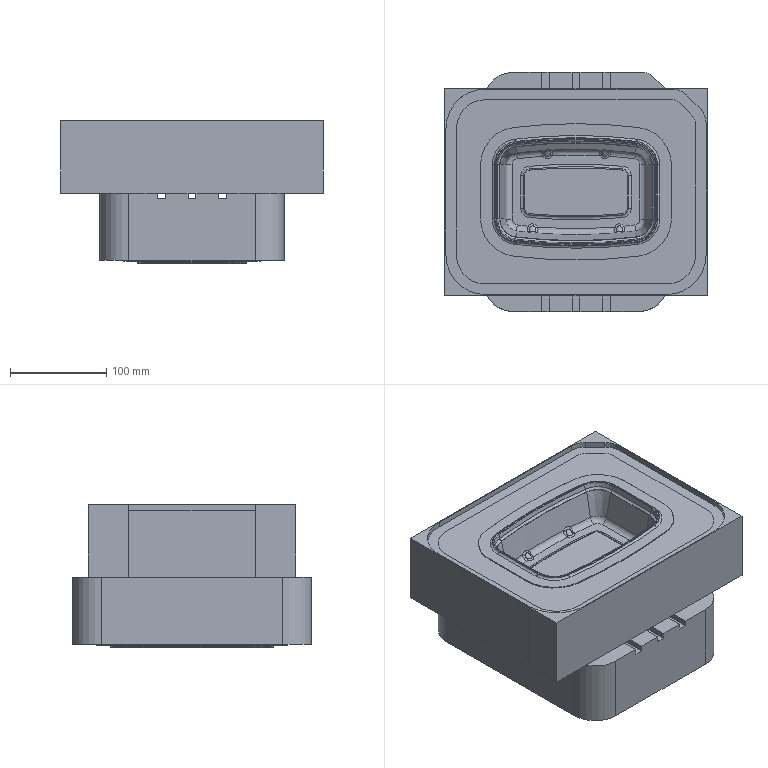NC program | NX | posted with a generic post | part box 272.387 x 248.388 x 148.5 mm
Lines 5839 to 6739 of 133013:
(CONTOUR_AREA_1 , TOOL : R2)
N11676 M6
N11678 G53
N11680 G17 G0 G90 X-11.083 Y-70.672 S8000 M3 M8
N11682 G43 Z133. H0
N11684 Z73.707
N11686 G94 G1 Z70.707 F4500.
N11688 X-11.776 Y-70.653
N11690 X-12.469 Y-70.629
N11692 X-13.16 Y-70.612
N11694 X-21.466 Y-70.357
N11696 X-22.535 Y-70.31
N11698 X-32.555 Y-69.794
N11700 X-33.592 Y-69.724
N11702 X-41.216 Y-69.179
N11704 X-43.287 Y-69.03
N11706 G3 X-50.565 Y-68.366 R5781.693
N11708 G1 X-54.029 Y-68.047
N11710 X-57.148 Y-67.701
N11712 X-64.761 Y-66.846
N11714 X-64.768 Y-66.841
N11716 X-65.111 Y-66.795
N11718 X-66.981 Y-66.5
N11720 X-67.876 Y-66.349
N11722 X-68.74 Y-66.153
N11724 X-70.174 Y-65.808
N11726 X-70.653 Y-65.686
N11728 X-70.998 Y-65.589
N11730 X-71.419 Y-65.461
N11732 X-71.695 Y-65.369
N11734 X-73.556 Y-64.768
N11736 X-73.771 Y-64.686
N11738 X-74.397 Y-64.432
N11740 X-74.812 Y-64.261
N11742 X-76.116 Y-63.729
N11744 X-76.539 Y-63.537
N11746 X-78.925 Y-62.343
N11748 X-79.525 Y-61.997
N11750 X-79.661 Y-61.916
N11752 X-81.252 Y-60.958
N11754 X-81.793 Y-60.612
N11756 X-83.741 Y-59.226
N11758 X-84.196 Y-58.88
N11760 X-84.856 Y-58.331
N11762 X-86.279 Y-57.148
N11764 X-88.419 Y-55.07
N11766 X-90.396 Y-52.834
N11768 X-92.129 Y-50.551
N11770 X-92.821 Y-49.485
N11772 X-93.237 Y-48.836
N11774 X-93.681 Y-48.143
N11776 X-93.888 Y-47.796
N11778 X-95.008 Y-45.718
N11780 X-95.189 Y-45.372
N11782 X-95.242 Y-45.265
N11784 X-96.285 Y-42.931
N11786 X-96.421 Y-42.601
N11788 X-96.551 Y-42.255
N11790 X-97.29 Y-40.177
N11792 X-97.322 Y-40.086
N11794 X-97.406 Y-39.831
N11796 X-97.6 Y-39.138
N11798 X-97.979 Y-37.752
N11800 X-98.162 Y-37.06
N11802 X-98.364 Y-36.069
N11804 X-98.707 Y-34.289
N11806 X-98.725 Y-34.247
N11808 X-99.073 Y-31.172
N11810 X-99.17 Y-28.747
N11812 X-99.189 Y-27.715
N11814 Y28.048
N11816 X-99.158 Y29.09
N11818 X-99.075 Y31.125
N11820 X-99.071 Y31.172
N11822 X-99.056 Y31.321
N11824 X-98.878 Y32.904
N11826 X-98.725 Y34.247
N11828 X-98.707 Y34.289
N11830 X-98.364 Y36.068
N11832 X-98.162 Y37.06
N11834 X-98.072 Y37.406
N11836 X-97.979 Y37.752
N11838 X-97.406 Y39.831
N11840 X-97.171 Y40.513
N11842 X-96.672 Y41.909
N11844 X-96.55 Y42.255
N11846 X-96.424 Y42.595
N11848 X-96.285 Y42.931
N11850 X-95.814 Y43.989
N11852 X-95.351 Y45.026
N11854 X-95.246 Y45.258
N11856 X-95.19 Y45.372
N11858 X-95.008 Y45.719
N11860 X-94.821 Y46.065
N11862 X-93.861 Y47.845
N11864 X-93.682 Y48.142
N11866 X-93.459 Y48.489
N11868 X-92.345 Y50.221
N11870 X-92.129 Y50.55
N11872 X-90.397 Y52.833
N11874 X-89.012 Y54.399
N11876 X-88.419 Y55.07
N11878 X-86.934 Y56.512
N11880 X-86.241 Y57.179
N11882 X-84.163 Y58.906
N11884 X-83.741 Y59.226
N11886 X-83.253 Y59.573
N11888 X-81.739 Y60.649
N11890 X-81.251 Y60.958
N11892 X-81.045 Y61.082
N11894 X-80.007 Y61.705
N11896 X-79.314 Y62.121
N11898 X-78.924 Y62.344
N11900 X-76.543 Y63.535
N11902 X-76.257 Y63.665
N11904 X-76.116 Y63.729
N11906 X-74.812 Y64.261
N11908 X-74.119 Y64.546
N11910 X-73.773 Y64.683
N11912 X-73.556 Y64.768
N11914 X-71.348 Y65.482
N11916 X-71.002 Y65.588
N11918 X-70.656 Y65.686
N11920 X-70.179 Y65.807
N11922 X-69.963 Y65.858
N11924 X-69.292 Y66.018
N11926 X-68.584 Y66.19
N11928 X-67.885 Y66.347
N11930 X-66.159 Y66.63
N11932 X-65.46 Y66.742
N11934 X-65.114 Y66.795
N11936 X-64.768 Y66.841
N11938 X-64.76 Y66.846
N11940 X-61.65 Y67.192
N11942 X-60.265 Y67.349
N11944 X-55.432 Y67.894
N11946 X-54.031 Y68.046
N11948 X-53.338 Y68.111
N11950 X-45.802 Y68.802
N11952 X-44.501 Y68.924
N11954 X-44.333 Y68.937
N11956 X-43.294 Y69.03
N11958 X-33.596 Y69.724
N11960 X-32.557 Y69.794
N11962 X-29.107 Y69.973
N11964 X-22.534 Y70.308
N11966 X-21.474 Y70.357
N11968 X-11.776 Y70.653
N11970 X-11.743 Y70.656
N11972 X-10.737 Y70.68
N11974 X-0.346 Y70.786
N11976 X0.
N11978 X0.345
N11980 X1.732 Y70.773
N11982 X3.803 Y70.751
N11984 X5.542 Y70.733
N11986 X6.927 Y70.721
N11988 X10.707 Y70.681
N11990 G2 X40.869 Y69.204 R522.773
N11992 G1 X43.287 Y69.03
N11994 G2 X53.684 Y68.08 R1157.552
N11996 G1 X54.377 Y68.01
N11998 X59.226 Y67.466
N12000 X60.954 Y67.273
N12002 X61.997 Y67.157
N12004 X62.688 Y67.078
N12006 X63.382 Y66.998
N12008 X64.761 Y66.846
N12010 X64.768 Y66.841
N12012 X65.111 Y66.795
N12014 X65.805 Y66.688
N12016 X66.5 Y66.576
N12018 X66.981 Y66.5
N12020 X67.876 Y66.349
N12022 X68.74 Y66.153
N12024 X70.174 Y65.808
N12026 X70.653 Y65.686
N12028 X70.998 Y65.589
N12030 X71.419 Y65.461
N12032 X73.556 Y64.768
N12034 X74.667 Y64.32
N12036 G2 X79.661 Y61.916 R33.441
N12038 G1 X81.252 Y60.958
N12040 X81.39 Y60.87
N12042 X81.793 Y60.612
N12044 X83.741 Y59.226
N12046 X83.817 Y59.168
N12048 X84.196 Y58.88
N12050 X85.862 Y57.495
N12052 X86.279 Y57.148
N12054 X88.419 Y55.07
N12056 X88.725 Y54.724
N12058 X90.396 Y52.834
N12060 X90.79 Y52.317
N12062 X92.129 Y50.551
N12064 X92.346 Y50.221
N12066 X92.79 Y49.532
N12068 X92.822 Y49.485
N12070 X93.237 Y48.836
N12072 X93.681 Y48.143
N12074 X93.888 Y47.796
N12076 X93.964 Y47.656 Z70.705
N12078 X94.072 Y47.455 Z70.707
N12080 X95.008 Y45.719
N12082 X95.19 Y45.372
N12084 X95.243 Y45.265
N12086 X96.285 Y42.931
N12088 X96.421 Y42.601
N12090 X96.551 Y42.255
N12092 X97.168 Y40.523
N12094 X97.406 Y39.831
N12096 X98.162 Y37.06
N12098 X98.364 Y36.069
N12100 X98.707 Y34.289
N12102 X98.725 Y34.247
N12104 X99.073 Y31.172
N12106 X99.158 Y29.094
N12108 X99.189 Y28.055
N12110 X99.185 Y-28.055
N12112 G2 X99.056 Y-31.321 R74.044
N12114 G1 X98.725 Y-34.247
N12116 X98.707 Y-34.289
N12118 X98.364 Y-36.068
N12120 X98.162 Y-37.06
N12122 X98.087 Y-37.352
N12124 X97.672 Y-38.88
N12126 X97.409 Y-39.821
N12128 X97.244 Y-40.311
N12130 X96.672 Y-41.909
N12132 X96.634 Y-42.021
N12134 X96.424 Y-42.595
N12136 X96.285 Y-42.931
N12138 X95.815 Y-43.987
N12140 X95.244 Y-45.262
N12142 X95.189 Y-45.372
N12144 X95.008 Y-45.719
N12146 X94.822 Y-46.065
N12148 X93.888 Y-47.796
N12150 X93.682 Y-48.142
N12152 X93.459 Y-48.489
N12154 X92.568 Y-49.875
N12156 X92.129 Y-50.55
N12158 X92.115 Y-50.568
N12160 X91.783 Y-51.006
N12162 X91.437 Y-51.464
N12164 X90.803 Y-52.299
N12166 X90.397 Y-52.833
N12168 X89.358 Y-54.008
N12170 X88.421 Y-55.067
N12172 X86.279 Y-57.148
N12174 X85.862 Y-57.495
N12176 G2 X81.392 Y-60.871 R37.735
N12178 G1 X79.526 Y-61.994
N12180 X78.925 Y-62.343
N12182 X76.543 Y-63.535
N12184 X76.115 Y-63.729
N12186 X73.773 Y-64.685
N12188 X73.556 Y-64.768
N12190 X72.045 Y-65.255
N12192 X71.43 Y-65.457
N12194 X71.002 Y-65.588
N12196 X70.656 Y-65.686
N12198 X70.18 Y-65.806
N12200 X68.931 Y-66.106
N12202 X68.745 Y-66.152
N12204 X67.885 Y-66.347
N12206 X66.983 Y-66.499
N12208 X66.5 Y-66.576
N12210 X65.807 Y-66.688
N12212 X65.114 Y-66.795
N12214 X64.768 Y-66.841
N12216 X64.76 Y-66.846
N12218 X61.65 Y-67.192
N12220 X60.958 Y-67.272
N12222 X59.919 Y-67.387
N12224 X59.226 Y-67.467
N12226 X58.187 Y-67.582
N12228 X57.494 Y-67.662
N12230 X56.455 Y-67.777
N12232 X55.869 Y-67.845
N12234 X55.52 Y-67.884
N12236 X54.377 Y-68.01
N12238 X53.684 Y-68.08
N12240 X44.333 Y-68.937
N12242 X43.294 Y-69.03
N12244 X42.601 Y-69.079
N12246 X32.903 Y-69.773
N12248 X29.44 Y-69.957
N12250 X25.284 Y-70.168
N12252 X24.591 Y-70.201
N12254 X23.898 Y-70.238
N12256 X22.874 Y-70.289
N12258 X22.534 Y-70.31
N12260 X21.474 Y-70.357
N12262 X11.43 Y-70.663
N12264 X10.737 Y-70.68
N12266 X10.506 Y-70.683
N12268 X8.659 Y-70.703
N12270 X0.347 Y-70.786
N12272 X-1.039 Y-70.78
N12274 X-10.737 Y-70.679
N12276 X-11.083 Y-70.672
N12278 Y-70.387
N12280 X-21.577 Y-70.067
N12282 X-22.513 Y-70.025
N12284 X-32.557 Y-69.508
N12286 X-39.83 Y-68.993
N12288 X-40.148 Y-68.971
N12290 X-41.186 Y-68.895
N12292 X-43.446 Y-68.73
N12294 X-45.986 Y-68.499
N12296 X-54.031 Y-67.759
N12298 X-56.027 Y-67.539
N12300 X-60.148 Y-67.076
N12302 X-61.393 Y-66.935
N12304 X-61.713 Y-66.902
N12306 G2 X-68.087 Y-66.009 R64.071
N12308 X-73.663 Y-64.422 R39.26
N12310 G1 X-74.223 Y-64.194
N12312 X-74.725 Y-63.989
N12314 G2 X-79.548 Y-61.651 R33.299
N12316 X-91.914 Y-50.358 R38.49
N12318 G1 X-92.605 Y-49.295
N12320 G2 X-96.529 Y-41.46 R35.482
N12322 G1 X-96.985 Y-40.189
N12324 X-97.081 Y-39.907
N12326 G2 X-98.214 Y-35.328 R35.034
N12328 G1 X-98.416 Y-34.289
N12330 X-98.459 Y-34.035
N12332 X-98.472 Y-33.943
N12334 X-98.784 Y-31.172
N12336 X-98.889 Y-28.58
N12338 X-98.904 Y-27.902
N12340 X-98.902 Y28.055
N12342 X-98.865 Y29.285
N12344 X-98.783 Y31.203
N12346 X-98.46 Y34.036
N12348 G2 X-97.081 Y39.901 R40.617
N12350 G1 X-96.978 Y40.198
N12352 X-96.802 Y40.7
N12354 G2 X-94.125 Y46.758 R33.961
N12356 G1 X-93.62 Y47.692
N12358 X-93.286 Y48.231
N12360 X-91.919 Y50.351
N12362 G2 X-70.33 Y65.474 R38.676
N12364 G1 X-70.019 Y65.551
N12366 X-69.371 Y65.707
N12368 G2 X-64.51 Y66.587 R34.841
N12370 G1 X-61.657 Y66.907
N12372 X-61.583 Y66.914
N12374 X-61.304 Y66.945
N12376 G2 X-36.401 Y69.237 R453.922
N12378 G1 X-35.328 Y69.315
N12380 X-34.981 Y69.339
N12382 X-32.557 Y69.508
N12384 G2 X10.82 Y70.393 R533.867
N12386 G1 X15.273 Y70.262
N12388 G2 X39.57 Y69.011 R454.953
N12390 G1 X40.148 Y68.971
N12392 X40.523 Y68.943
N12394 G2 X61.713 Y66.902 R454.097
N12396 G1 X62.023 Y66.867
N12398 X63.382 Y66.711
N12400 G2 X67.885 Y66.054 R50.215
N12402 X76.431 Y63.27 R39.532
N12404 X91.917 Y50.354 R38.732
N12406 G1 X92.605 Y49.295
N12408 G2 X98.148 Y35.674 R37.937
N12410 G1 X98.417 Y34.289
N12412 X98.46 Y34.036
N12414 X98.784 Y31.172
N12416 X98.878 Y28.915
N12418 X98.904 Y27.902
N12420 X98.902 Y-28.055
N12422 X98.877 Y-28.926
N12424 X98.783 Y-31.203
N12426 X98.459 Y-34.035
N12428 G2 X96.221 Y-42.32 R40.059
N12430 X92.228 Y-49.875 R37.191
N12432 G1 X91.919 Y-50.351
N12434 X90.179 Y-52.646
N12436 X88.326 Y-54.745
N12438 X88.003 Y-55.079
N12440 X87.656 Y-55.416
N12442 G2 X74.517 Y-64.075 R37.871
N12444 G1 X74.224 Y-64.195
N12446 X73.663 Y-64.422
N12448 X73.426 Y-64.51
N12450 X72.459 Y-64.823
N12452 X71.76 Y-65.049
N12454 X71.364 Y-65.179
N12456 X71.248 Y-65.214
N12458 X70.656 Y-65.388
N12460 X70.385 Y-65.461
N12462 X70.331 Y-65.475
N12464 X70.02 Y-65.551
N12466 X68.577 Y-65.898
N12468 G2 X64.51 Y-66.587 R37.613
N12470 G1 X61.657 Y-66.907
N12472 X61.582 Y-66.914
N12474 X60.958 Y-66.985
N12476 G2 X40.544 Y-68.941 R450.136
N12478 G1 X40.177 Y-68.969
N12480 X39.757 Y-68.997
N12482 X32.674 Y-69.5
N12484 X28.747 Y-69.705
N12486 X22.903 Y-70.002
N12488 X22.517 Y-70.025
N12490 X21.82 Y-70.056
N12492 X20.781 Y-70.091
N12494 X12.843 Y-70.334
N12496 X10.65 Y-70.396
N12498 X0. Y-70.502
N12500 X-10.82 Y-70.393
N12502 X-11.083 Y-70.387
N12504 Y-70.102
N12506 X-21.636 Y-69.779
N12508 X-23.552 Y-69.685
N12510 X-32.512 Y-69.225
N12512 X-40.177 Y-68.683
N12514 X-43.501 Y-68.439
N12516 X-44.679 Y-68.335
N12518 X-54.031 Y-67.473
N12520 X-57.089 Y-67.134
N12522 X-64.56 Y-66.292
N12524 G2 X-73.521 Y-64.17 R41.197
N12526 X-91.658 Y-50.221 R38.444
N12528 G1 X-92.338 Y-49.182
N12530 X-93.202 Y-47.831
N12532 X-93.515 Y-47.288
N12534 X-94.665 Y-45.148
N12536 X-95.308 Y-43.724
N12538 G2 X-98.125 Y-34.289 R37.617
N12540 G1 X-98.161 Y-34.086
N12542 G2 X-98.618 Y-27.963 R40.788
N12544 G1 X-98.615 Y28.149
N12546 G2 X-98.46 Y31.518 R77.107
N12548 X-97.539 Y37.192 R35.328
N12550 X-95.701 Y42.84 R39.307
N12552 X-92.56 Y48.836 R36.752
N12554 X-85.895 Y56.712 R37.84
N12556 X-65.039 Y66.229 R38.365
N12558 G1 X-64.639 Y66.282
N12560 G2 X10.88 Y70.106 R532.641
N12562 G1 X15.288 Y69.976
N12564 X21.636 Y69.779
N12566 G2 X43.294 Y68.456 R559.26
N12568 G1 X45.994 Y68.213
N12570 G2 X65.114 Y66.218 R500.357
N12572 X70.309 Y65.185 R37.681
N12574 X73.521 Y64.17 R32.159
N12576 X93.515 Y47.287 R38.331
N12578 X98.591 Y28.974 R38.203
N12580 G1 X98.618 Y27.963
N12582 X98.616 Y-28.149
N12584 X98.586 Y-29.094
N12586 G2 X97.538 Y-37.192 R36.316
N12588 X93.305 Y-47.66 R38.64
N12590 X89.799 Y-52.646 R39.677
N12592 X86.173 Y-56.456 R37.052
N12594 X65.039 Y-66.228 R38.449
N12596 G1 X64.639 Y-66.282
N12598 G2 X0.092 Y-70.217 R540.463
N12600 G1 X-8.659 Y-70.133
N12602 X-11.083 Y-70.102
N12604 X-11.076 Y-69.817
N12606 X-21.694 Y-69.491
N12608 X-29.786 Y-69.082
N12610 X-32.555 Y-68.937
N12612 X-43.238 Y-68.175
N12614 X-44.829 Y-68.035
N12616 X-53.973 Y-67.192
N12618 X-58.533 Y-66.685
N12620 X-64.612 Y-65.998
N12622 G2 X-73.546 Y-63.854 R38.916
N12624 X-91.504 Y-49.942 R38.116
N12626 G1 X-92.129 Y-48.98
N12628 G2 X-97.528 Y-35.878 R37.067
N12630 X-98.333 Y-28.024 R38.449
N12632 G1 X-98.332 Y28.086
N12634 X-98.312 Y28.747
N12636 G2 X-96.433 Y40.029 R37.083
N12638 X-64.571 Y66.003 R38.089
N12640 X43.294 Y68.171 R532.489
N12642 G1 X46.097 Y67.917
N12644 X53.682 Y67.221
N12646 X55.416 Y67.036
N12648 X64.612 Y65.998
N12650 G2 X73.546 Y63.854 R38.887
N12652 X91.437 Y50.042 R38.131
N12654 G1 X92.129 Y48.98
N12656 G2 X97.528 Y35.878 R37.056
N12658 X98.323 Y28.401 R37.333
N12660 G1 X98.333 Y28.024
N12662 X98.332 Y-28.086
N12664 X98.324 Y-28.401
N12666 X98.312 Y-28.799
N12668 G2 X97.893 Y-33.943 R40.122
N12670 G1 X97.871 Y-34.089
N12672 X97.457 Y-36.234
N12674 G2 X92.129 Y-48.98 R37.548
N12676 G1 X91.437 Y-50.038
N12678 G2 X87.973 Y-54.278 R40.986
N12680 X64.571 Y-66.003 R38.122
N12682 X29.44 Y-69.101 R523.114
N12684 X10.527 Y-69.827 R478.814
N12686 G1 X0.03 Y-69.933
N12688 X-10.6 Y-69.826
N12690 X-10.94 Y-69.82
N12692 X-11.076 Y-69.817
N12694 X-11.068 Y-69.532
N12696 X-21.42 Y-69.217
N12698 G2 X-58.442 Y-66.409 R514.424
N12700 G1 X-64.421 Y-65.735
N12702 G2 X-75.64 Y-62.69 R38.52
N12704 X-91.204 Y-49.875 R37.832
N12706 G1 X-91.883 Y-48.836
N12708 G2 X-97.277 Y-35.674 R36.78
N12710 G1 X-97.565 Y-34.183
N12712 X-97.607 Y-33.943
N12714 G2 X-98.047 Y-28.089 R39.97
N12716 G1 X-98.048 Y28.021
N12718 G2 X-97.913 Y31.276 R45.935
N12720 X-96.467 Y38.956 R35.912
N12722 G1 X-96.33 Y39.44
N12724 G2 X-95.246 Y42.453 R73.943
N12726 X-89.63 Y51.953 R38.041
N12728 X-73.651 Y63.504 R37.754
N12730 X-64.503 Y65.725 R38.644
N12732 X13.693 Y69.455 R530.504
N12734 X46.755 Y67.57 R495.456
N12736 X65.27 Y65.617 R434.821
N12738 X97.565 Y34.183 R37.729
N12740 G1 X97.607 Y33.943
N12742 X97.616 Y33.887
N12744 X97.923 Y31.172
N12746 X97.949 Y30.757
N12748 X98.017 Y29.094
N12750 X98.047 Y28.089
N12752 X98.049 Y-28.02
N12754 G2 X97.913 Y-31.276 R46.903
N12756 X96.466 Y-38.957 R38.469
N12758 X92.962 Y-47.104 R36.701
N12760 G1 X92.822 Y-47.354
N12762 G2 X91.09 Y-50.03 R71.844
N12764 X64.503 Y-65.725 R37.832
N12766 X22.257 Y-69.18 R538.667
N12768 G1 X21.531 Y-69.213
N12770 G2 X-11.068 Y-69.532 R537.912
N12772 G1 X-11.06 Y-69.247
N12774 X-21.473 Y-68.93
N12776 X-23.461 Y-68.833
N12778 X-32.356 Y-68.377
N12780 X-35.272 Y-68.176
N12782 G2 X-58.496 Y-66.116 R486.59
N12784 G1 X-64.41 Y-65.45
N12786 G2 X-78.318 Y-61.047 R38.223
N12788 X-93.906 Y-44.75 R37.454
N12790 G1 X-94.563 Y-43.294
N12792 G2 X-96.978 Y-35.721 R35.934
N12794 G1 X-97.324 Y-33.91
N12796 X-97.642 Y-31.143
N12798 G2 X-97.762 Y-28.055 R103.283
N12800 G1 Y28.055
N12802 G2 X-97.635 Y31.208 R95.138
N12804 X-96.71 Y36.982 R35.154
N12806 G1 X-96.119 Y39.138
N12808 X-96.052 Y39.371
N12810 G2 X-95.019 Y42.255 R77.519
N12812 X-73.023 Y63.44 R37.639
N12814 X-64.318 Y65.461 R39.061
N12816 X10.721 Y69.255 R532.311
N12818 G1 X15.325 Y69.12
N12820 G2 X45.573 Y67.393 R504.84
N12822 G1 X53.818 Y66.634
N12824 X55.382 Y66.466
N12826 X64.41 Y65.45
N12828 G2 X78.275 Y61.07 R38.206
N12830 X97.36 Y33.632 R37.453
N12832 G1 X97.5 Y32.402
N12834 G2 X97.74 Y28.817 R25.703
N12836 G1 X97.76 Y28.144
N12838 X97.762 Y28.055
N12840 Y-28.055
N12842 G2 X96.71 Y-36.982 R38.006
N12844 X81.046 Y-59.388 R37.45
N12846 X64.835 Y-65.394 R37.73
N12848 X29.49 Y-68.528 R513.606
N12850 G1 X22.193 Y-68.898
N12852 G2 X-11.06 Y-69.247 R528.151
N12854 G1 X-11.081 Y-68.961
N12856 X-21.474 Y-68.645
N12858 G2 X-54.031 Y-66.326 R535.764
N12860 G1 X-58.531 Y-65.825
N12862 X-64.42 Y-65.161
N12864 G2 X-73.102 Y-63.109 R39.742
N12866 X-90.744 Y-49.539 R37.29
N12868 X-93.622 Y-44.68 R40.427
N12870 X-96.684 Y-35.738 R36.386
N12872 X-97.464 Y-28.541 R34.735
N12874 G1 X-97.478 Y-27.862
N12876 X-97.476 Y28.055
N12878 X-97.437 Y29.328
N12880 G2 X-97.04 Y33.88 R32.842
N12882 X-90.978 Y49.182 R37.588
N12884 X-87.356 Y53.685 R37.229
N12886 X-65.173 Y65.056 R37.142
N12888 G1 X-64.368 Y65.168
N12890 G2 X-32.719 Y68.069 R537.621
N12892 G1 X-26.508 Y68.393
N12894 X-22.13 Y68.615
N12896 X-21.474 Y68.645
N12898 G2 X10.735 Y68.97 R532.128
N12900 G1 X15.215 Y68.838
N12902 X21.474 Y68.645
N12904 G2 X55.414 Y66.175 R532.578
N12906 G1 X64.42 Y65.161
N12908 G2 X75.352 Y62.191 R37.931
N12910 X90.744 Y49.54 R37.378
N12912 X93.622 Y44.68 R40.53
N12914 X97.476 Y28.055 R37.734
N12916 G1 X97.477 Y-28.055
N12918 G2 X97.04 Y-33.881 R40.605
N12920 X89.012 Y-51.806 R37.234
N12922 X82.731 Y-57.841 R37.953
N12924 X77.87 Y-60.958 R36.322
N12926 X65.173 Y-65.055 R37.121
N12928 G1 X64.368 Y-65.167
N12930 G2 X29.442 Y-68.245 R515.836
N12932 X10.739 Y-68.97 R469.788
N12934 G1 X0. Y-69.077
N12936 X-10.735 Y-68.97
N12938 X-11.081 Y-68.961
N12940 X-11.083 Y-68.676
N12942 X-21.596 Y-68.354
N12944 X-29.785 Y-67.94
N12946 X-32.796 Y-67.778
N12948 X-42.818 Y-67.063
N12950 X-43.46 Y-67.012
N12952 X-53.927 Y-66.05
N12954 X-58.533 Y-65.538
N12956 X-64.514 Y-64.861
N12958 G2 X-77.922 Y-60.612 R37.297
N12960 X-97.177 Y-28.6 R36.873
N12962 G1 X-97.193 Y-27.923
N12964 X-97.191 Y28.055
N12966 G2 X-97.064 Y31.172 R50.895
N12968 X-94.675 Y41.562 R36.762
N12970 G1 X-94.554 Y41.888
N12972 X-94.545 Y41.909
N12974 X-94.093 Y42.948
N12976 G2 X-92.129 Y46.839 R37.749
N12978 X-90.393 Y49.528 R63.015
N12980 X-65.116 Y64.776 R36.91
N12982 G1 X-64.301 Y64.888
N12984 G2 X-32.654 Y67.788 R535.275
N12986 G1 X-26.444 Y68.111
N12988 X-21.82 Y68.344
N12990 X-21.474 Y68.359
N12992 G2 X10.841 Y68.682 R534.356
N12994 G1 X16.797 Y68.504
N12996 X21.596 Y68.354
N12998 G2 X46.064 Y66.776 R529.889
N13000 G1 X53.927 Y66.049
N13002 X57.045 Y65.704
N13004 X64.514 Y64.861
N13006 G2 X75.85 Y61.651 R37.326
N13008 X89.204 Y51.106 R36.752
N13010 X97.166 Y28.935 R36.726
N13012 G1 X97.193 Y27.923
N13014 X97.192 Y-28.055
N13016 G2 X97.064 Y-31.172 R53.256
N13018 X66.753 Y-64.514 R36.887
N13020 G1 X65.807 Y-64.667
N13022 X65.115 Y-64.776
N13024 X64.301 Y-64.888
N13026 X54.159 Y-66.025
N13028 G2 X20.781 Y-68.38 R537.912
N13030 X-11.083 Y-68.676 R522.207
N13032 G1 Y-68.391
N13034 G2 X-65.114 Y-64.488 R530.419
N13036 X-90.193 Y-49.324 R36.614
N13038 X-95.803 Y-37.06 R36.525
N13040 G1 X-95.894 Y-36.713
N13042 X-95.939 Y-36.531
N13044 X-96.143 Y-35.532
N13046 G2 X-96.908 Y-27.984 R36.867
N13048 G1 X-96.905 Y28.127
N13050 G2 X-96.502 Y33.596 R40.415
N13052 G1 X-96.483 Y33.745
N13054 G2 X-93.315 Y43.987 R36.478
N13056 G1 X-93.168 Y44.303
N13058 G2 X-91.634 Y47.104 R54.293
N13060 X-64.768 Y64.539 R36.601
N13062 G1 X-64.234 Y64.609
N13064 X-54.092 Y65.746
N13066 G2 X-24.594 Y67.919 R517.587
N13068 G1 X-21.474 Y68.074
N13070 X-11.083 Y68.391
N13072 X-10.391 Y68.404
N13074 X0. Y68.508
N13076 X10.737 Y68.399
N13078 X14.957 Y68.276
N13080 X21.655 Y68.066
N13082 G2 X46.001 Y66.495 R506.823
N13084 G1 X53.667 Y65.79
N13086 X56.109 Y65.523
N13088 X64.421 Y64.585
N13090 G2 X78.161 Y60.151 R37.342
N13092 X93.161 Y44.326 R36.696
N13094 G1 X93.782 Y42.948
N13096 G2 X96.144 Y35.533 R34.523
N13098 X96.879 Y28.994 R33.866
N13100 G1 X96.908 Y27.984
N13102 X96.906 Y-28.127
N13104 G2 X95.986 Y-36.32 R37.528
N13106 X90.522 Y-48.836 R36.629
N13108 X64.768 Y-64.539 R36.65
N13110 G1 X64.075 Y-64.627
N13112 G2 X-11.083 Y-68.391 R535.947
N13114 G1 X-11.076 Y-68.106
N13116 X-21.474 Y-67.789
N13118 G2 X-64.311 Y-64.312 R531.593
N13120 X-78.171 Y-59.815 R37.012
N13122 X-95.893 Y-35.328 R36.258
N13124 X-96.623 Y-28.055 R36.503
N13126 G1 X-96.622 Y28.055
N13128 X-96.59 Y29.094
N13130 G2 X-95.709 Y36.251 R35.42
N13132 X-67.456 Y63.812 R36.369
N13134 G1 X-66.617 Y63.958
N13136 X-64.768 Y64.251
N13138 X-64.075 Y64.341
N13140 X-54.078 Y65.461
N13142 X-52.645 Y65.597
N13144 X-43.343 Y66.45
N13146 X-38.587 Y66.796
N13148 X-32.56 Y67.223
N13150 X-24.591 Y67.634
N13152 X-21.474 Y67.788
N13154 X-10.857 Y68.111
N13156 X-0.008 Y68.223
N13158 X10.737 Y68.114
N13160 X15.758 Y67.966
N13162 G2 X48.143 Y66.013 R497.621
N13164 G1 X53.682 Y65.502
N13166 X55.762 Y65.275
N13168 X64.421 Y64.298
N13170 G2 X75.851 Y61.014 R36.38
N13172 X93.055 Y43.874 R36.124
N13174 X95.893 Y35.328 R35.676
N13176 X96.59 Y29.094 R31.695
N13178 G1 X96.623 Y28.055
N13180 Y-28.055
N13182 X96.603 Y-28.747
N13184 G2 X86.502 Y-53.338 R36.233
N13186 X64.768 Y-64.25 R36.313
N13188 G1 X64.075 Y-64.34
N13190 G2 X38.533 Y-66.799 R496.529
N13192 X0.008 Y-68.223 R513.343
N13194 G1 X-10.737 Y-68.114
N13196 X-10.961 Y-68.109
N13198 X-11.076 Y-68.106
N13200 X-11.068 Y-67.821
N13202 X-21.44 Y-67.505
N13204 G2 X-43.292 Y-66.168 R604.612
N13206 G1 X-44.58 Y-66.054
N13208 X-53.684 Y-65.215
N13210 X-55.96 Y-64.966
N13212 X-64.364 Y-64.018
N13214 G2 X-80.281 Y-58.187 R36.53
N13216 X-95.593 Y-35.377 R36.007
N13218 X-96.337 Y-28.055 R36.275
N13220 G1 Y28.055
N13222 G2 X-96.194 Y31.263 R76.288
N13224 X-92.683 Y43.987 R35.758
N13226 X-69.616 Y63.008 R36.086
N13228 X-64.099 Y64.051 R37.079
N13230 G1 X-54.736 Y65.102
N13232 X-53.338 Y65.248
N13234 X-43.296 Y66.168
N13236 X-35.674 Y66.718
N13238 X-32.46 Y66.943
N13240 X-24.518 Y67.352
N13242 X-21.51 Y67.502
N13244 G2 X10.737 Y67.829 R531.459
N13246 G1 X16.53 Y67.657
N13248 X21.44 Y67.505
N13250 G2 X65.114 Y63.91 R521.64
N13252 X93.79 Y41.491 R36.044
N13254 X96.235 Y30.775 R36.653
N13256 G1 X96.248 Y30.479
N13258 X96.304 Y29.116
N13260 X96.336 Y28.108
N13262 X96.337 Y28.055
N13264 Y-28.055
N13266 G2 X72.805 Y-61.997 R36.081
N13268 X64.099 Y-64.051 R37.118
N13270 G1 X54.031 Y-65.179
N13272 G2 X-11.068 Y-67.821 R531.454
N13274 G1 X-11.06 Y-67.536
N13276 X-21.471 Y-67.219
N13278 X-24.917 Y-67.046
N13280 G2 X-57.148 Y-64.546 R492.605
N13282 G1 X-64.375 Y-63.729
N13284 G2 X-72.387 Y-61.847 R37.092
N13286 X-87.973 Y-50.833 R36.115
N13288 X-96.052 Y-28.055 R35.976
N13290 G1 X-96.051 Y28.055
N13292 G2 X-95.918 Y31.172 R53.233
N13294 G1 X-95.642 Y33.583
N13296 G2 X-91.09 Y46.355 R36.692
N13298 X-64.831 Y63.666 R35.791
N13300 G1 X-64.421 Y63.724
N13302 X-64.078 Y63.767
N13304 X-54.031 Y64.892
N13306 X-52.744 Y65.016
N13308 X-43.294 Y65.882
N13310 X-37.406 Y66.308
N13312 X-32.557 Y66.651
N13314 X-26.004 Y66.991
N13316 X-21.477 Y67.218
N13318 G2 X10.736 Y67.544 R531.09
N13320 G1 X15.445 Y67.405
N13322 X21.471 Y67.219
N13324 X24.245 Y67.081
N13326 X31.518 Y66.709
N13328 X33.25 Y66.605
N13330 X42.947 Y65.91
N13332 X45.869 Y65.649
N13334 X53.684 Y64.928
N13336 X55.703 Y64.708
N13338 X64.374 Y63.729
N13340 G2 X72.909 Y61.651 R36.524
N13342 X87.937 Y50.877 R36.08
N13344 X96.02 Y29.094 R35.716
N13346 G1 X96.049 Y28.164
N13348 X96.051 Y28.055
N13350 X96.052 Y-28.055
N13352 G2 X95.918 Y-31.172 R75.786
N13354 X64.421 Y-63.724 R35.8
N13356 X-11.06 Y-67.536 R532.125
N13358 G1 X-11.053 Y-67.251
N13360 G2 X-64.15 Y-63.47 R530.431
N13362 X-79.913 Y-57.747 R35.769
N13364 X-90.505 Y-46.758 R35.041
N13366 G1 X-90.733 Y-46.4
N13368 G2 X-95.767 Y-27.883 R35.981
N13370 G1 X-95.765 Y28.055
N13372 X-95.726 Y29.307
N13374 G2 X-92.377 Y43.294 R34.925
N13376 X-63.965 Y63.492 R35.553
N13378 X-25.979 Y66.707 R513.028
N13380 G1 X-21.474 Y66.933
N13382 G2 X10.776 Y67.258 R530.631
N13384 G1 X17.311 Y67.062
N13386 X21.557 Y66.93
N13388 G2 X64.15 Y63.47 R531.038
N13390 X77.236 Y59.36 R35.877
N13392 X89.369 Y48.516 R35.406
N13394 X92.052 Y43.987 R40.573
N13396 X95.741 Y28.896 R35.398
N13398 G1 X95.767 Y27.883
N13400 X95.766 Y-28.055
N13402 X95.739 Y-28.948
N13404 G2 X85.293 Y-53.338 R35.324
N13406 X64.075 Y-63.479 R35.596
N13408 X-11.053 Y-67.251 R529.869
N13410 G1 X-11.045 Y-66.966
N13412 G2 X-64.213 Y-63.174 R529.256
N13414 X-77.315 Y-58.992 R36.038
N13416 X-95.466 Y-28.62 R35.197
N13418 G1 X-95.482 Y-27.944
N13420 X-95.478 Y28.169
N13422 X-95.443 Y29.243
N13424 G2 X-92.974 Y41.216 R34.639
N13426 X-63.898 Y63.213 R35.268
N13428 X-26.149 Y66.413 R516.927
N13430 G1 X-21.474 Y66.647
N13432 X-11.083 Y66.965
N13434 X-9.556 Y66.988
N13436 X0. Y67.082
N13438 X10.861 Y66.971
N13440 X17.394 Y66.774
N13442 X21.615 Y66.641
N13444 X31.504 Y66.139
N13446 X33.138 Y66.041
N13448 X43.154 Y65.321
N13450 X47.917 Y64.889
N13452 X53.684 Y64.355
N13454 X56.266 Y64.071
N13456 X64.213 Y63.174
N13458 G2 X78.093 Y58.534 R35.617
N13460 X94.731 Y35.328 R35.058
N13462 X95.454 Y28.955 R33.268
N13464 G1 X95.482 Y27.944
N13466 X95.479 Y-28.168
N13468 G2 X94.373 Y-36.894 R35.882
N13470 X64.075 Y-63.192 R35.218